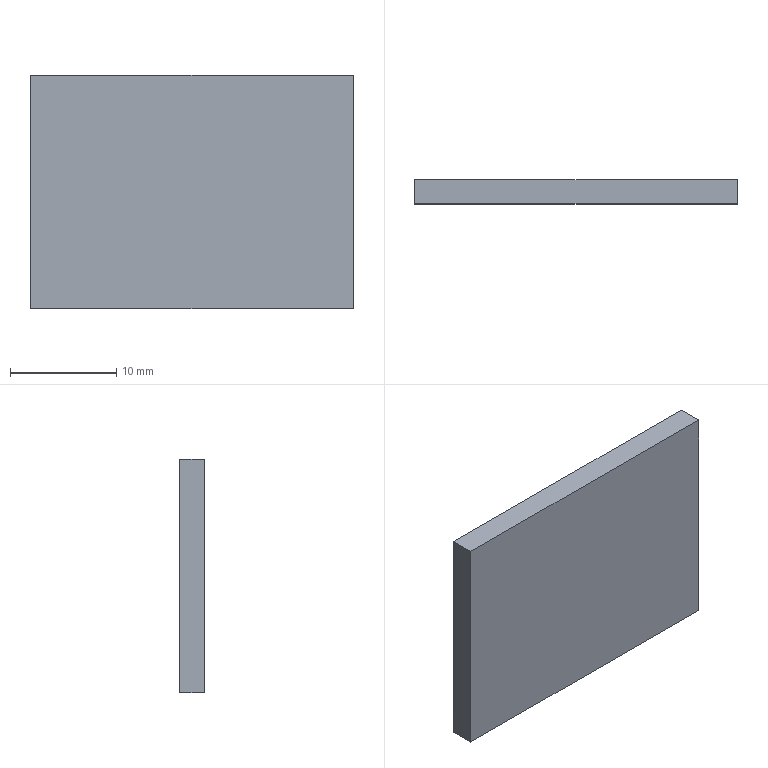Part | SolidWorks | features FlatPattern 1, SMBaseFlange 1, SheetMetal 1 | 1 solid | 6 faces | box 30.4 x 2.3 x 22 mm | volume 1538 mm3 | plane 6
STEP:
#1=CARTESIAN_POINT('',(15.2,0.,11.));
#2=VERTEX_POINT('',#1);
#3=CARTESIAN_POINT('',(15.2,0.,-11.));
#4=VERTEX_POINT('',#3);
#5=CARTESIAN_POINT('',(15.2,0.,-11.));
#6=DIRECTION('',(0.,0.,-1.));
#7=VECTOR('',#6,1000.);
#8=LINE('',#5,#7);
#9=EDGE_CURVE('',#2,#4,#8,.T.);
#10=ORIENTED_EDGE('',*,*,#9,.T.);
#11=CARTESIAN_POINT('',(15.2,2.3,-11.));
#12=VERTEX_POINT('',#11);
#13=CARTESIAN_POINT('',(15.2,2.3,-11.));
#14=DIRECTION('',(0.,-1.,0.));
#15=VECTOR('',#14,1000.);
#16=LINE('',#13,#15);
#17=EDGE_CURVE('',#12,#4,#16,.T.);
#18=ORIENTED_EDGE('',*,*,#17,.F.);
#19=CARTESIAN_POINT('',(15.2,2.3,11.));
#20=VERTEX_POINT('',#19);
#21=CARTESIAN_POINT('',(15.2,2.3,-11.));
#22=DIRECTION('',(0.,0.,-1.));
#23=VECTOR('',#22,1000.);
#24=LINE('',#21,#23);
#25=EDGE_CURVE('',#20,#12,#24,.T.);
#26=ORIENTED_EDGE('',*,*,#25,.F.);
#27=CARTESIAN_POINT('',(15.2,2.3,11.));
#28=DIRECTION('',(0.,-1.,0.));
#29=VECTOR('',#28,1000.);
#30=LINE('',#27,#29);
#31=EDGE_CURVE('',#20,#2,#30,.T.);
#32=ORIENTED_EDGE('',*,*,#31,.T.);
#33=EDGE_LOOP('',(#10,#18,#26,#32));
#34=FACE_OUTER_BOUND('',#33,.T.);
#35=CARTESIAN_POINT('',(15.2,2.3,-11.));
#36=DIRECTION('',(-1.,0.,0.));
#37=DIRECTION('',(0.,0.,1.));
#38=AXIS2_PLACEMENT_3D('',#35,#36,#37);
#39=PLANE('',#38);
#40=ADVANCED_FACE('',(#34),#39,.F.);
#41=CARTESIAN_POINT('',(-15.2,0.,-11.));
#42=VERTEX_POINT('',#41);
#43=CARTESIAN_POINT('',(-15.2,0.,-11.));
#44=DIRECTION('',(-1.,0.,0.));
#45=VECTOR('',#44,1000.);
#46=LINE('',#43,#45);
#47=EDGE_CURVE('',#4,#42,#46,.T.);
#48=ORIENTED_EDGE('',*,*,#47,.T.);
#49=CARTESIAN_POINT('',(-15.2,2.3,-11.));
#50=VERTEX_POINT('',#49);
#51=CARTESIAN_POINT('',(-15.2,2.3,-11.));
#52=DIRECTION('',(0.,-1.,0.));
#53=VECTOR('',#52,1000.);
#54=LINE('',#51,#53);
#55=EDGE_CURVE('',#50,#42,#54,.T.);
#56=ORIENTED_EDGE('',*,*,#55,.F.);
#57=CARTESIAN_POINT('',(-15.2,2.3,-11.));
#58=DIRECTION('',(-1.,0.,0.));
#59=VECTOR('',#58,1000.);
#60=LINE('',#57,#59);
#61=EDGE_CURVE('',#12,#50,#60,.T.);
#62=ORIENTED_EDGE('',*,*,#61,.F.);
#63=ORIENTED_EDGE('',*,*,#17,.T.);
#64=EDGE_LOOP('',(#48,#56,#62,#63));
#65=FACE_OUTER_BOUND('',#64,.T.);
#66=CARTESIAN_POINT('',(-15.2,2.3,-11.));
#67=DIRECTION('',(0.,0.,1.));
#68=DIRECTION('',(1.,0.,0.));
#69=AXIS2_PLACEMENT_3D('',#66,#67,#68);
#70=PLANE('',#69);
#71=ADVANCED_FACE('',(#65),#70,.F.);
#72=CARTESIAN_POINT('',(-15.2,0.,11.));
#73=VERTEX_POINT('',#72);
#74=CARTESIAN_POINT('',(-15.2,0.,-11.));
#75=DIRECTION('',(0.,0.,1.));
#76=VECTOR('',#75,1000.);
#77=LINE('',#74,#76);
#78=EDGE_CURVE('',#42,#73,#77,.T.);
#79=ORIENTED_EDGE('',*,*,#78,.T.);
#80=CARTESIAN_POINT('',(-15.2,2.3,11.));
#81=VERTEX_POINT('',#80);
#82=CARTESIAN_POINT('',(-15.2,2.3,11.));
#83=DIRECTION('',(0.,-1.,0.));
#84=VECTOR('',#83,1000.);
#85=LINE('',#82,#84);
#86=EDGE_CURVE('',#81,#73,#85,.T.);
#87=ORIENTED_EDGE('',*,*,#86,.F.);
#88=CARTESIAN_POINT('',(-15.2,2.3,-11.));
#89=DIRECTION('',(0.,0.,1.));
#90=VECTOR('',#89,1000.);
#91=LINE('',#88,#90);
#92=EDGE_CURVE('',#50,#81,#91,.T.);
#93=ORIENTED_EDGE('',*,*,#92,.F.);
#94=ORIENTED_EDGE('',*,*,#55,.T.);
#95=EDGE_LOOP('',(#79,#87,#93,#94));
#96=FACE_OUTER_BOUND('',#95,.T.);
#97=CARTESIAN_POINT('',(-15.2,2.3,-11.));
#98=DIRECTION('',(1.,0.,0.));
#99=DIRECTION('',(0.,0.,-1.));
#100=AXIS2_PLACEMENT_3D('',#97,#98,#99);
#101=PLANE('',#100);
#102=ADVANCED_FACE('',(#96),#101,.F.);
#103=CARTESIAN_POINT('',(-15.2,0.,11.));
#104=DIRECTION('',(1.,0.,0.));
#105=VECTOR('',#104,1000.);
#106=LINE('',#103,#105);
#107=EDGE_CURVE('',#73,#2,#106,.T.);
#108=ORIENTED_EDGE('',*,*,#107,.T.);
#109=ORIENTED_EDGE('',*,*,#31,.F.);
#110=CARTESIAN_POINT('',(-15.2,2.3,11.));
#111=DIRECTION('',(1.,0.,0.));
#112=VECTOR('',#111,1000.);
#113=LINE('',#110,#112);
#114=EDGE_CURVE('',#81,#20,#113,.T.);
#115=ORIENTED_EDGE('',*,*,#114,.F.);
#116=ORIENTED_EDGE('',*,*,#86,.T.);
#117=EDGE_LOOP('',(#108,#109,#115,#116));
#118=FACE_OUTER_BOUND('',#117,.T.);
#119=CARTESIAN_POINT('',(-15.2,2.3,11.));
#120=DIRECTION('',(0.,0.,-1.));
#121=DIRECTION('',(-1.,0.,0.));
#122=AXIS2_PLACEMENT_3D('',#119,#120,#121);
#123=PLANE('',#122);
#124=ADVANCED_FACE('',(#118),#123,.F.);
#125=ORIENTED_EDGE('',*,*,#25,.T.);
#126=ORIENTED_EDGE('',*,*,#61,.T.);
#127=ORIENTED_EDGE('',*,*,#92,.T.);
#128=ORIENTED_EDGE('',*,*,#114,.T.);
#129=EDGE_LOOP('',(#125,#126,#127,#128));
#130=FACE_OUTER_BOUND('',#129,.T.);
#131=CARTESIAN_POINT('',(0.,2.3,0.));
#132=DIRECTION('',(0.,1.,0.));
#133=DIRECTION('',(0.,0.,1.));
#134=AXIS2_PLACEMENT_3D('',#131,#132,#133);
#135=PLANE('',#134);
#136=ADVANCED_FACE('',(#130),#135,.T.);
#137=ORIENTED_EDGE('',*,*,#9,.F.);
#138=ORIENTED_EDGE('',*,*,#107,.F.);
#139=ORIENTED_EDGE('',*,*,#78,.F.);
#140=ORIENTED_EDGE('',*,*,#47,.F.);
#141=EDGE_LOOP('',(#137,#138,#139,#140));
#142=FACE_OUTER_BOUND('',#141,.T.);
#143=CARTESIAN_POINT('',(0.,0.,0.));
#144=DIRECTION('',(0.,1.,0.));
#145=DIRECTION('',(0.,0.,1.));
#146=AXIS2_PLACEMENT_3D('',#143,#144,#145);
#147=PLANE('',#146);
#148=ADVANCED_FACE('',(#142),#147,.F.);
#149=CLOSED_SHELL('',(#40,#71,#102,#124,#136,#148));
#150=MANIFOLD_SOLID_BREP('',#149);
#151=CARTESIAN_POINT('',(0.,0.,0.));
#152=DIRECTION('',(0.,0.,1.));
#153=DIRECTION('',(1.,0.,0.));
#154=AXIS2_PLACEMENT_3D('',#151,#152,#153);
#155=(LENGTH_UNIT()NAMED_UNIT(*)SI_UNIT(.MILLI.,.METRE.));
#156=UNCERTAINTY_MEASURE_WITH_UNIT(LENGTH_MEASURE(0.00001),#155,'','');
#157=(NAMED_UNIT(*)PLANE_ANGLE_UNIT()SI_UNIT($,.RADIAN.));
#158=(NAMED_UNIT(*)SI_UNIT($,.STERADIAN.)SOLID_ANGLE_UNIT());
#159=(GEOMETRIC_REPRESENTATION_CONTEXT(3)GLOBAL_UNCERTAINTY_ASSIGNED_CONTEXT((#156))GLOBAL_UNIT_ASSIGNED_CONTEXT((#155,#157,#158))REPRESENTATION_CONTEXT('',''));
#160=ADVANCED_BREP_SHAPE_REPRESENTATION('',(#150,#154),#159);